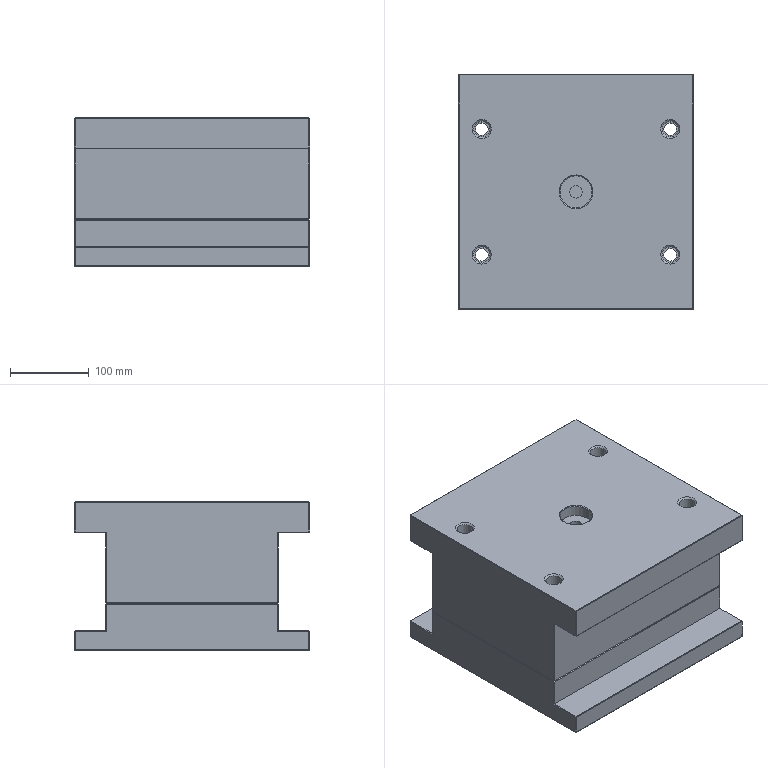NC program | NX | posted with a generic post | part box 300 x 300 x 190 mm
Whole program:
N10 G17 G21 G94 G90
(PLANAR_MILL_COPY_1 , TOOL : D6A45)
N12 T07 M6
N14 G54
N16 G17 G0 G90 X110. Y-79.134 S7500 M3
N18 G43 Z30. H7
N20 Z0.
N22 G94 G1 Z-1.5 F1250.
N24 G3 X109.5 Y-80. R1.
N26 X120. Y-90.5 R10.5
N28 X109.5 Y-80. R-10.5
N30 X110. Y-80.866 R1.
N32 G1 Z0.
N34 G0 Z30.
N36 Y80.866
N38 Z0.
N40 G1 Z-1.5
N42 G3 X109.5 Y80. R1.
N44 X120. Y69.5 R10.5
N46 X109.5 Y80. R-10.5
N48 X110. Y79.134 R1.
N50 G1 Z0.
N52 G0 Z30.
N54 X-130. Y80.866
N56 Z0.
N58 G1 Z-1.5
N60 G3 X-130.5 Y80. R1.
N62 X-120. Y69.5 R10.5
N64 X-130.5 Y80. R-10.5
N66 X-130. Y79.134 R1.
N68 G1 Z0.
N70 G0 Z30.
N72 Y-79.134
N74 Z0.
N76 G1 Z-1.5
N78 G3 X-130.5 Y-80. R1.
N80 X-120. Y-90.5 R10.5
N82 X-130.5 Y-80. R-10.5
N84 X-130. Y-80.866 R1.
N86 G1 Z0.
N88 G0 Z30.
N90 M5
N92 M2